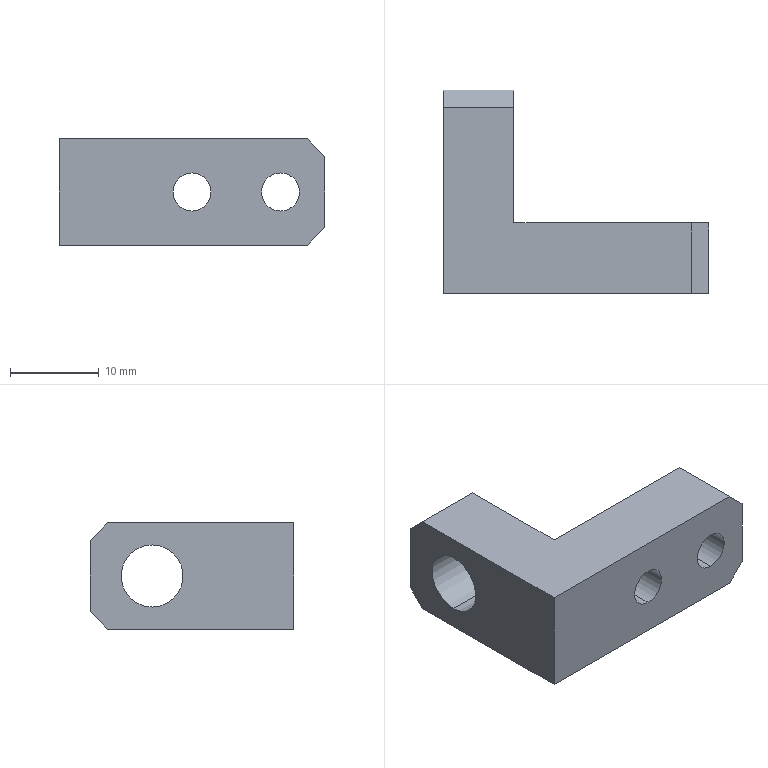Part | STEP file | PN_0055 Mount electronic clip limit mounting block A | 1 solid | 24 faces | box 30 x 23 x 12 mm | volume 3387 mm3 | plane 14 | cylinder 10 | commonest cylinder face diameters 4.3 x4 8 x4 7 x2